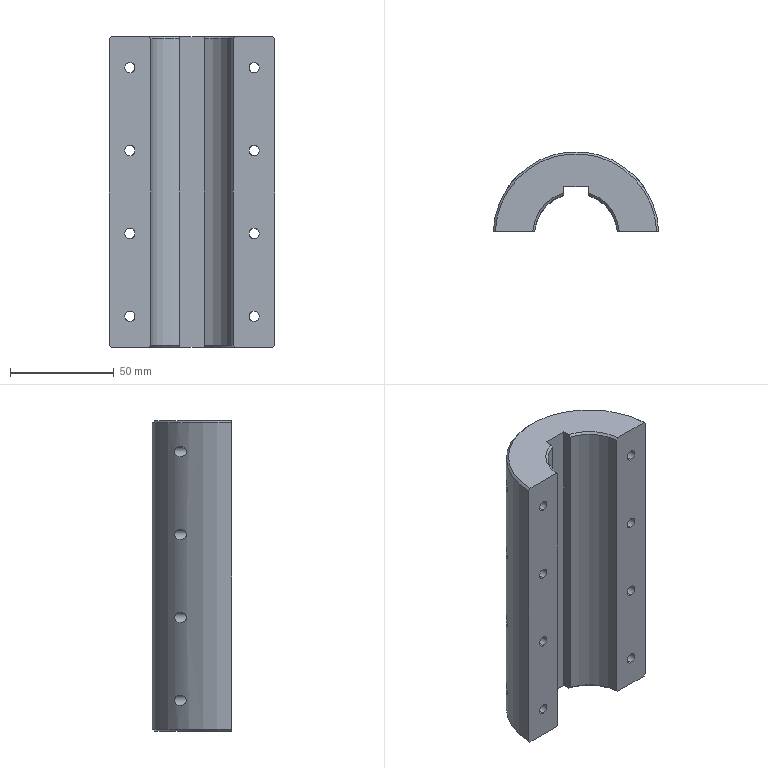Part | SolidWorks | features Chamfer 1, Extrusion 1, HoleWzd 1, ICE 1, LPattern 1 | 1 solid | 32 faces | box 79.944 x 38.5 x 150 mm | volume 263173 mm3 | cylinder 19 | plane 7 | cone 6 | commonest cylinder face diameters 5 x16 40 x2 80 x1